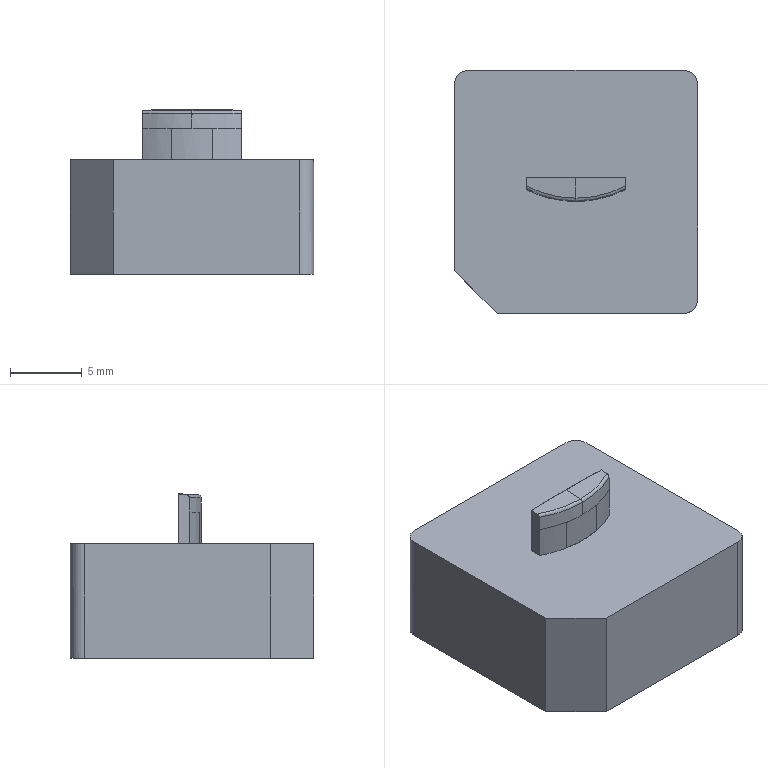NC program | PowerMill | posted with a generic post | part box 17 x 17 x 11.498 mm
Lines 2037 to 3902 of 31087, first 1642 of 1866 lines:
N2134 M6
N2135 S18000 M03
N2136 G00 G90 X0.0 Y0.0
N2137 G43 Z9.7979 H2
N2138
N2139 G05 P10000 R4
N2140 X-1.4386 Y3.9377
N2141 Z0.7981
N2142 G01 Z-0.4019 F3600.0
N2143 X-1.4484 Y3.918 F6000.0
N2144 G03 X-1.3599 Y3.6524 I0.1771 J-0.0885
N2145 G01 X0.0 Y2.9724
N2146 X3.1723
N2147 X3.6604 Y2.9618
N2148 X4.1484 Y2.848
N2149 X4.4884 Y2.6843
N2150 X4.6365 Y2.5854
N2151 X5.0359 Y2.1962
N2152 X5.1246 Y2.0722
N2153 X5.3138 Y1.7082
N2154 X5.4386 Y1.2201
N2155 X5.4548 Y0.244
N2156 X5.4013 Y-0.244
N2157 X5.2178 Y-0.7321
N2158 X5.1246 Y-0.89
N2159 X4.852 Y-1.2201
N2160 X4.6365 Y-1.4029
N2161 X4.1484 Y-1.6736
N2162 X3.6604 Y-1.8871
N2163 X2.7944 Y-2.1962
N2164 X2.1962 Y-2.3549
N2165 X1.7082 Y-2.4558
N2166 X0.7321 Y-2.5782
N2167 X-0.244 Y-2.6041
N2168 X-1.2201 Y-2.5297
N2169 X-2.1962 Y-2.3537
N2170 X-3.1723 Y-2.0713
N2171 X-4.0749 Y-1.7082
N2172 X-4.6365 Y-1.4029
N2173 X-4.852 Y-1.2201
N2174 X-5.1246 Y-0.89
N2175 X-5.2178 Y-0.7321
N2176 X-5.4013 Y-0.244
N2177 X-5.4548 Y0.244
N2178 X-5.4386 Y1.2201
N2179 X-5.3138 Y1.7082
N2180 X-5.1246 Y2.0722
N2181 X-5.0359 Y2.1962
N2182 X-4.6365 Y2.5854
N2183 X-4.4884 Y2.6843
N2184 X-4.1484 Y2.848
N2185 X-3.6604 Y2.9618
N2186 X-3.1723 Y2.9724
N2187 X0.0
N2188 X-1.4386 Y3.9377 Z-0.5918
N2189 X-1.4484 Y3.918
N2190 G03 X-1.3599 Y3.6524 I0.1771 J-0.0885
N2191 G01 X0.0 Y2.9724
N2192 X3.1723
N2193 X3.6604 Y2.9618
N2194 X4.1484 Y2.848
N2195 X4.4884 Y2.6843
N2196 X4.6365 Y2.5854
N2197 X5.0359 Y2.1962
N2198 X5.1246 Y2.0723
N2199 X5.3138 Y1.7082
N2200 X5.4387 Y1.2201
N2201 X5.4548 Y0.244
N2202 X5.4054 Y-0.244
N2203 X5.2275 Y-0.7321
N2204 X5.1246 Y-0.9098
N2205 X4.8736 Y-1.2201
N2206 X4.6365 Y-1.4248
N2207 X4.1484 Y-1.6942
N2208 X3.6604 Y-1.9098
N2209 X2.8607 Y-2.1962
N2210 X1.7082 Y-2.4809
N2211 X0.7321 Y-2.605
N2212 X-0.244 Y-2.6289
N2213 X-1.2201 Y-2.5538
N2214 X-2.1962 Y-2.3796
N2215 X-3.1723 Y-2.0983
N2216 X-4.1201 Y-1.7082
N2217 X-4.6365 Y-1.4248
N2218 X-4.8736 Y-1.2201
N2219 X-5.1246 Y-0.9098
N2220 X-5.2275 Y-0.7321
N2221 X-5.4054 Y-0.244
N2222 X-5.4548 Y0.244
N2223 X-5.4387 Y1.2201
N2224 X-5.3138 Y1.7082
N2225 X-5.1246 Y2.0723
N2226 X-5.0359 Y2.1962
N2227 X-4.6365 Y2.5854
N2228 X-4.4884 Y2.6843
N2229 X-4.1484 Y2.848
N2230 X-3.6604 Y2.9618
N2231 X-3.1723 Y2.9724
N2232 X0.0
N2233 X-1.4386 Y3.9377 Z-0.7817
N2234 X-1.4484 Y3.918
N2235 G03 X-1.3599 Y3.6524 I0.1771 J-0.0885
N2236 G01 X0.0 Y2.9725
N2237 X3.1723
N2238 X3.6604 Y2.9618
N2239 X4.1484 Y2.848
N2240 X4.4884 Y2.6843
N2241 X4.6365 Y2.5854
N2242 X5.0359 Y2.1962
N2243 X5.1246 Y2.0723
N2244 X5.3138 Y1.7082
N2245 X5.4387 Y1.2201
N2246 X5.4548 Y0.244
N2247 X5.4084 Y-0.244
N2248 X5.2325 Y-0.7321
N2249 X5.1246 Y-0.919
N2250 X4.8815 Y-1.2201
N2251 X4.6365 Y-1.4323
N2252 X4.1484 Y-1.7022
N2253 X3.6604 Y-1.9188
N2254 X2.8763 Y-2.1962
N2255 X2.6843 Y-2.2555
N2256 X1.7082 Y-2.4878
N2257 X0.7321 Y-2.6129
N2258 X0.244 Y-2.6332
N2259 X0.0001 Y-2.6253
N2260 X-0.244 Y-2.6288
N2261 X-0.3653 Y-2.6195
N2262 X-0.3706 Y-2.6194
N2263 X-0.7321 Y-2.6113
N2264 X-1.1344 Y-2.5604
N2265 X-1.2188 Y-2.554
N2266 X-1.302 Y-2.5392
N2267 X-1.7082 Y-2.4878
N2268 X-2.1962 Y-2.3842
N2269 X-3.1723 Y-2.1053
N2270 X-4.1354 Y-1.7082
N2271 X-4.6365 Y-1.4323
N2272 X-4.8815 Y-1.2201
N2273 X-5.1246 Y-0.919
N2274 X-5.2325 Y-0.7321
N2275 X-5.4084 Y-0.244
N2276 X-5.4548 Y0.244
N2277 X-5.4387 Y1.2201
N2278 X-5.3138 Y1.7082
N2279 X-5.1246 Y2.0723
N2280 X-5.0359 Y2.1962
N2281 X-4.6365 Y2.5854
N2282 X-4.4884 Y2.6843
N2283 X-4.1484 Y2.848
N2284 X-3.6604 Y2.9618
N2285 X-3.1723 Y2.9725
N2286 X0.0
N2287 X-1.4386 Y3.9377 Z-0.9715
N2288 X-1.4484 Y3.918
N2289 G03 X-1.3599 Y3.6524 I0.1771 J-0.0885
N2290 G01 X0.0 Y2.9725
N2291 X3.1723
N2292 X3.6604 Y2.9618
N2293 X4.1484 Y2.848
N2294 X4.4884 Y2.6843
N2295 X4.6365 Y2.5854
N2296 X5.0359 Y2.1962
N2297 X5.1246 Y2.0723
N2298 X5.3138 Y1.7082
N2299 X5.4387 Y1.2201
N2300 X5.4548 Y0.244
N2301 X5.41 Y-0.244
N2302 X5.2374 Y-0.7321
N2303 X5.1246 Y-0.9264
N2304 X4.8886 Y-1.2201
N2305 X4.6365 Y-1.4397
N2306 X4.1512 Y-1.7082
N2307 X3.6604 Y-1.9256
N2308 X2.899 Y-2.1962
N2309 X2.6843 Y-2.2629
N2310 X1.7082 Y-2.4946
N2311 X0.7321 Y-2.6196
N2312 X0.244 Y-2.6407
N2313 X-0.7321 Y-2.6183
N2314 X-1.7082 Y-2.4947
N2315 X-2.1962 Y-2.3909
N2316 X-3.1723 Y-2.1123
N2317 X-4.1507 Y-1.7082
N2318 X-4.6365 Y-1.4397
N2319 X-4.8886 Y-1.2201
N2320 X-5.1246 Y-0.9264
N2321 X-5.2374 Y-0.7321
N2322 X-5.41 Y-0.244
N2323 X-5.4548 Y0.244
N2324 X-5.4387 Y1.2201
N2325 X-5.3138 Y1.7082
N2326 X-5.1246 Y2.0723
N2327 X-5.0359 Y2.1962
N2328 X-4.6365 Y2.5854
N2329 X-4.4884 Y2.6843
N2330 X-4.1484 Y2.848
N2331 X-3.6604 Y2.9618
N2332 X-3.1723 Y2.9725
N2333 X0.0
N2334 X-1.4386 Y3.9377 Z-1.1614
N2335 X-1.4484 Y3.918
N2336 G03 X-1.3599 Y3.6524 I0.1771 J-0.0885
N2337 G01 X0.0 Y2.9725
N2338 X3.1723
N2339 X3.6604 Y2.9618
N2340 X4.1484 Y2.848
N2341 X4.4884 Y2.6843
N2342 X4.6365 Y2.5854
N2343 X5.0359 Y2.1962
N2344 X5.1246 Y2.0723
N2345 X5.3138 Y1.7082
N2346 X5.4387 Y1.2201
N2347 X5.4548 Y0.244
N2348 X5.4116 Y-0.244
N2349 X5.2411 Y-0.7321
N2350 X5.1246 Y-0.9339
N2351 X4.8958 Y-1.2201
N2352 X4.6365 Y-1.4471
N2353 X4.167 Y-1.7082
N2354 X3.6604 Y-1.9325
N2355 X2.9221 Y-2.1962
N2356 X2.6843 Y-2.2704
N2357 X1.7082 Y-2.5015
N2358 X0.7321 Y-2.6262
N2359 X0.244 Y-2.6482
N2360 X-0.7321 Y-2.6254
N2361 X-1.7082 Y-2.5015
N2362 X-2.1962 Y-2.3978
N2363 X-3.1723 Y-2.1193
N2364 X-4.1484 Y-1.7168
N2365 X-4.6365 Y-1.4471
N2366 X-4.8958 Y-1.2201
N2367 X-5.1246 Y-0.9339
N2368 X-5.2411 Y-0.7321
N2369 X-5.4116 Y-0.244
N2370 X-5.4548 Y0.244
N2371 X-5.4387 Y1.2201
N2372 X-5.3138 Y1.7082
N2373 X-5.1246 Y2.0723
N2374 X-5.0359 Y2.1962
N2375 X-4.6365 Y2.5854
N2376 X-4.4884 Y2.6843
N2377 X-4.1484 Y2.848
N2378 X-3.6604 Y2.9618
N2379 X-3.1723 Y2.9725
N2380 X0.0
N2381 X-1.4386 Y3.9377 Z-1.3513
N2382 X-1.4484 Y3.918
N2383 G03 X-1.3599 Y3.6524 I0.1771 J-0.0885
N2384 G01 X0.0 Y2.9725
N2385 X3.1723
N2386 X3.6604 Y2.9618
N2387 X4.1484 Y2.848
N2388 X4.4884 Y2.6843
N2389 X4.6365 Y2.5855
N2390 X5.036 Y2.1962
N2391 X5.1246 Y2.0723
N2392 X5.3138 Y1.7082
N2393 X5.4387 Y1.2201
N2394 X5.4548 Y0.244
N2395 X5.4131 Y-0.244
N2396 X5.2449 Y-0.7321
N2397 X5.1246 Y-0.9413
N2398 X4.9029 Y-1.2201
N2399 X4.6365 Y-1.4545
N2400 X4.1828 Y-1.7082
N2401 X3.6604 Y-1.9394
N2402 X2.9463 Y-2.1962
N2403 X2.6843 Y-2.2778
N2404 X1.7082 Y-2.5084
N2405 X1.2201 Y-2.5815
N2406 X0.8795 Y-2.6073
N2407 X0.7321 Y-2.6262
N2408 X0.4866 Y-2.6372
N2409 X0.4835 Y-2.6374
N2410 X0.244 Y-2.6557
N2411 X-0.7321 Y-2.6325
N2412 X-1.7082 Y-2.5084
N2413 X-2.1962 Y-2.4046
N2414 X-3.1723 Y-2.1262
N2415 X-4.1828 Y-1.7082
N2416 X-4.6365 Y-1.4545
N2417 X-4.9029 Y-1.2201
N2418 X-5.1246 Y-0.9413
N2419 X-5.2449 Y-0.7321
N2420 X-5.4131 Y-0.244
N2421 X-5.4548 Y0.244
N2422 X-5.4387 Y1.2201
N2423 X-5.3138 Y1.7082
N2424 X-5.1246 Y2.0723
N2425 X-5.036 Y2.1962
N2426 X-4.6365 Y2.5855
N2427 X-4.4884 Y2.6843
N2428 X-4.1484 Y2.848
N2429 X-3.6604 Y2.9618
N2430 X-3.1723 Y2.9725
N2431 X0.0
N2432 X-1.4386 Y3.9377 Z-1.5412
N2433 X-1.4484 Y3.9181
N2434 G03 X-1.3599 Y3.6524 I0.1771 J-0.0886
N2435 G01 X0.0 Y2.9725
N2436 X3.1723
N2437 X3.6604 Y2.9618
N2438 X4.1484 Y2.848
N2439 X4.4884 Y2.6843
N2440 X4.6365 Y2.5855
N2441 X5.036 Y2.1962
N2442 X5.1246 Y2.0723
N2443 X5.3138 Y1.7082
N2444 X5.4387 Y1.2201
N2445 X5.4548 Y0.244
N2446 X5.4142 Y-0.244
N2447 X5.2473 Y-0.7321
N2448 X5.1246 Y-0.9464
N2449 X4.9078 Y-1.2201
N2450 X4.6365 Y-1.4596
N2451 X4.1938 Y-1.7082
N2452 X3.6604 Y-1.9463
N2453 X2.9714 Y-2.1962
N2454 X2.6843 Y-2.2836
N2455 X1.7082 Y-2.5141
N2456 X1.451 Y-2.5469
N2457 X1.2866 Y-2.5739
N2458 X1.1206 Y-2.589
N2459 X0.7321 Y-2.6385
N2460 X0.3461 Y-2.6478
N2461 X0.24 Y-2.6557
N2462 X0.1337 Y-2.653
N2463 X-0.244 Y-2.6621
N2464 X-0.5986 Y-2.6356
N2465 X-0.7311 Y-2.6325
N2466 X-0.8626 Y-2.6158
N2467 X-1.2201 Y-2.5891
N2468 X-1.5521 Y-2.5282
N2469 X-1.7082 Y-2.5084
N2470 X-2.0065 Y-2.4449
N2471 X-2.0093 Y-2.4444
N2472 X-2.1962 Y-2.4101
N2473 X-3.1723 Y-2.1315
N2474 X-4.194 Y-1.7082
N2475 X-4.6365 Y-1.4596
N2476 X-4.9078 Y-1.2201
N2477 X-5.1246 Y-0.9464
N2478 X-5.2473 Y-0.7321
N2479 X-5.4142 Y-0.244
N2480 X-5.4548 Y0.244
N2481 X-5.4387 Y1.2201
N2482 X-5.3138 Y1.7082
N2483 X-5.1246 Y2.0723
N2484 X-5.036 Y2.1962
N2485 X-4.6365 Y2.5855
N2486 X-4.4884 Y2.6843
N2487 X-4.1484 Y2.848
N2488 X-3.6604 Y2.9618
N2489 X-3.1723 Y2.9725
N2490 X0.0
N2491 X-1.4386 Y3.9377 Z-1.7311
N2492 X-1.4484 Y3.9181
N2493 G03 X-1.3599 Y3.6524 I0.1771 J-0.0886
N2494 G01 X0.0 Y2.9725
N2495 X3.1723
N2496 X3.6604 Y2.9618
N2497 X4.1484 Y2.848
N2498 X4.4884 Y2.6843
N2499 X4.6365 Y2.5855
N2500 X5.036 Y2.1962
N2501 X5.1246 Y2.0723
N2502 X5.3138 Y1.7082
N2503 X5.4387 Y1.2201
N2504 X5.4548 Y0.244
N2505 X5.4142 Y-0.244
N2506 X5.2473 Y-0.7321
N2507 X5.1246 Y-0.9465
N2508 X4.9079 Y-1.2201
N2509 X4.6365 Y-1.4596
N2510 X4.1939 Y-1.7082
N2511 X3.6604 Y-1.947
N2512 X2.9714 Y-2.1962
N2513 X2.6843 Y-2.2837
N2514 X1.7082 Y-2.5141
N2515 X1.4483 Y-2.5472
N2516 X1.2858 Y-2.574
N2517 X1.1218 Y-2.5888
N2518 X0.7321 Y-2.6385
N2519 X0.345 Y-2.6479
N2520 X0.2401 Y-2.6557
N2521 X0.1349 Y-2.653
N2522 X-0.244 Y-2.6621
N2523 X-0.5998 Y-2.6355
N2524 X-0.7311 Y-2.6324
N2525 X-0.8615 Y-2.6159
N2526 X-1.2201 Y-2.5891
N2527 X-1.5532 Y-2.528
N2528 X-1.5586 Y-2.5273
N2529 X-1.7082 Y-2.5083
N2530 X-1.9515 Y-2.4558
N2531 X-2.1962 Y-2.4101
N2532 X-3.1723 Y-2.1315
N2533 X-3.6604 Y-1.9456
N2534 X-4.194 Y-1.7082
N2535 X-4.6365 Y-1.4596
N2536 X-4.9079 Y-1.2201
N2537 X-5.1246 Y-0.9465
N2538 X-5.2473 Y-0.7321
N2539 X-5.4142 Y-0.244
N2540 X-5.4548 Y0.244
N2541 X-5.4387 Y1.2201
N2542 X-5.3138 Y1.7082
N2543 X-5.1246 Y2.0723
N2544 X-5.036 Y2.1962
N2545 X-4.6365 Y2.5855
N2546 X-4.4884 Y2.6843
N2547 X-4.1484 Y2.848
N2548 X-3.6604 Y2.9618
N2549 X-3.1723 Y2.9725
N2550 X0.0
N2551 X-1.4386 Y3.9377 Z-1.921
N2552 X-1.4484 Y3.9181
N2553 G03 X-1.3599 Y3.6524 I0.1771 J-0.0886
N2554 G01 X0.0 Y2.9725
N2555 X3.1723
N2556 X3.6604 Y2.9618
N2557 X4.1484 Y2.848
N2558 X4.4884 Y2.6843
N2559 X4.6365 Y2.5855
N2560 X5.036 Y2.1962
N2561 X5.1246 Y2.0723
N2562 X5.3138 Y1.7082
N2563 X5.4387 Y1.2201
N2564 X5.4548 Y0.244
N2565 X5.4142 Y-0.244
N2566 X5.2473 Y-0.7321
N2567 X5.1246 Y-0.9465
N2568 X4.9079 Y-1.2201
N2569 X4.6365 Y-1.4596
N2570 X4.1939 Y-1.7082
N2571 X3.6604 Y-1.9472
N2572 X2.9714 Y-2.1962
N2573 X2.6843 Y-2.2837
N2574 X1.7082 Y-2.5141
N2575 X1.4456 Y-2.5476
N2576 X1.285 Y-2.574
N2577 X1.1229 Y-2.5887
N2578 X0.7321 Y-2.6385
N2579 X0.3438 Y-2.6479
N2580 X0.2401 Y-2.6556
N2581 X0.1361 Y-2.6529
N2582 X-0.244 Y-2.6621
N2583 X-0.6009 Y-2.6354
N2584 X-0.7311 Y-2.6324
N2585 X-0.8604 Y-2.616
N2586 X-1.2201 Y-2.5891
N2587 X-1.5543 Y-2.5278
N2588 X-1.5596 Y-2.5271
N2589 X-1.7082 Y-2.5083
N2590 X-1.9515 Y-2.4558
N2591 X-2.1962 Y-2.4101
N2592 X-3.1723 Y-2.1316
N2593 X-3.6604 Y-1.946
N2594 X-4.194 Y-1.7082
N2595 X-4.6365 Y-1.4596
N2596 X-4.9079 Y-1.2201
N2597 X-5.1246 Y-0.9465
N2598 X-5.2473 Y-0.7321
N2599 X-5.4142 Y-0.244
N2600 X-5.4548 Y0.244
N2601 X-5.4387 Y1.2201
N2602 X-5.3138 Y1.7082
N2603 X-5.1246 Y2.0723
N2604 X-5.036 Y2.1962
N2605 X-4.6365 Y2.5855
N2606 X-4.4884 Y2.6843
N2607 X-4.1484 Y2.848
N2608 X-3.6604 Y2.9618
N2609 X-3.1723 Y2.9725
N2610 X0.0
N2611 X-1.4386 Y3.9377 Z-2.1109
N2612 X-1.4484 Y3.9181
N2613 G03 X-1.3598 Y3.6524 I0.1771 J-0.0886
N2614 G01 X0.0 Y2.9725
N2615 X3.1723
N2616 X3.6604 Y2.9618
N2617 X4.1484 Y2.848
N2618 X4.4884 Y2.6843
N2619 X4.6365 Y2.5855
N2620 X5.036 Y2.1962
N2621 X5.1246 Y2.0723
N2622 X5.3138 Y1.7082
N2623 X5.4387 Y1.2201
N2624 X5.4548 Y0.244
N2625 X5.4142 Y-0.244
N2626 X5.2474 Y-0.7321
N2627 X5.1246 Y-0.9465
N2628 X4.9079 Y-1.2201
N2629 X4.6365 Y-1.4596
N2630 X4.1939 Y-1.7082
N2631 X3.6604 Y-1.9472
N2632 X2.9714 Y-2.1962
N2633 X2.6843 Y-2.2837
N2634 X1.7082 Y-2.5141
N2635 X1.4429 Y-2.5479
N2636 X1.2842 Y-2.574
N2637 X1.1241 Y-2.5886
N2638 X0.7321 Y-2.6385
N2639 X0.3427 Y-2.648
N2640 X0.2402 Y-2.6556
N2641 X0.1374 Y-2.6529
N2642 X-0.244 Y-2.6621
N2643 X-0.6021 Y-2.6353
N2644 X-0.7311 Y-2.6323
N2645 X-0.8592 Y-2.6161
N2646 X-1.2201 Y-2.5891
N2647 X-1.5553 Y-2.5276
N2648 X-1.5607 Y-2.527
N2649 X-1.7082 Y-2.5082
N2650 X-1.9515 Y-2.4557
N2651 X-2.1962 Y-2.4102
N2652 X-3.1723 Y-2.1316
N2653 X-3.6604 Y-1.9464
N2654 X-4.194 Y-1.7082
N2655 X-4.6365 Y-1.4596
N2656 X-4.9079 Y-1.2201
N2657 X-5.1246 Y-0.9465
N2658 X-5.2474 Y-0.7321
N2659 X-5.4142 Y-0.244
N2660 X-5.4548 Y0.244
N2661 X-5.4387 Y1.2201
N2662 X-5.3138 Y1.7082
N2663 X-5.1246 Y2.0723
N2664 X-5.036 Y2.1962
N2665 X-4.6365 Y2.5855
N2666 X-4.4884 Y2.6843
N2667 X-4.1484 Y2.848
N2668 X-3.6604 Y2.9618
N2669 X-3.1723 Y2.9725
N2670 X0.0
N2671 X-1.4386 Y3.9377 Z-2.3008
N2672 X-1.4484 Y3.9181
N2673 G03 X-1.3598 Y3.6524 I0.1771 J-0.0886
N2674 G01 X0.0 Y2.9725
N2675 X3.1723
N2676 X3.6604 Y2.9618
N2677 X4.1484 Y2.8481
N2678 X4.4884 Y2.6843
N2679 X4.6365 Y2.5855
N2680 X5.036 Y2.1962
N2681 X5.1246 Y2.0723
N2682 X5.3138 Y1.7082
N2683 X5.4387 Y1.2201
N2684 X5.4548 Y0.244
N2685 X5.4142 Y-0.244
N2686 X5.2474 Y-0.7321
N2687 X5.1246 Y-0.9465
N2688 X4.9079 Y-1.2201
N2689 X4.6365 Y-1.4597
N2690 X4.1939 Y-1.7082
N2691 X3.6604 Y-1.9472
N2692 X2.9714 Y-2.1962
N2693 X2.7316 Y-2.2708
N2694 X2.4876 Y-2.3302
N2695 X2.1962 Y-2.4109
N2696 X1.9509 Y-2.4562
N2697 X1.7082 Y-2.514
N2698 X1.4631 Y-2.545
N2699 X1.2201 Y-2.5891
N2700 X0.9755 Y-2.6074
N2701 X0.7321 Y-2.6385
N2702 X0.4878 Y-2.6441
N2703 X0.244 Y-2.6619
N2704 X0.0 Y-2.6561
N2705 X-0.244 Y-2.6621
N2706 X-0.4878 Y-2.6441
N2707 X-0.7321 Y-2.6384
N2708 X-0.9755 Y-2.6074
N2709 X-1.2201 Y-2.589
N2710 X-1.4631 Y-2.5449
N2711 X-1.7082 Y-2.5141
N2712 X-1.951 Y-2.4564
N2713 X-2.1962 Y-2.4101
N2714 X-2.4388 Y-2.3417
N2715 X-2.6843 Y-2.285
N2716 X-2.9262 Y-2.2015
N2717 X-3.1723 Y-2.1315
N2718 X-3.6468 Y-1.9515
N2719 X-3.6604 Y-1.9468
N2720 X-4.194 Y-1.7082
N2721 X-4.6365 Y-1.4597
N2722 X-4.9079 Y-1.2201
N2723 X-5.1246 Y-0.9465
N2724 X-5.2474 Y-0.7321
N2725 X-5.4142 Y-0.244
N2726 X-5.4548 Y0.244
N2727 X-5.4387 Y1.2201
N2728 X-5.3138 Y1.7082
N2729 X-5.1246 Y2.0723
N2730 X-5.036 Y2.1962
N2731 X-4.6365 Y2.5855
N2732 X-4.4884 Y2.6843
N2733 X-4.1484 Y2.8481
N2734 X-3.6604 Y2.9618
N2735 X-3.1723 Y2.9725
N2736 X0.0
N2737 X-1.4386 Y3.9377 Z-2.4907
N2738 X-1.4484 Y3.9181
N2739 G03 X-1.3598 Y3.6524 I0.1771 J-0.0886
N2740 G01 X0.0 Y2.9725
N2741 X3.1723
N2742 X3.6604 Y2.9618
N2743 X4.1484 Y2.8481
N2744 X4.4884 Y2.6843
N2745 X4.6365 Y2.5855
N2746 X5.036 Y2.1962
N2747 X5.1246 Y2.0723
N2748 X5.3138 Y1.7082
N2749 X5.4387 Y1.2201
N2750 X5.4548 Y0.244
N2751 X5.4142 Y-0.244
N2752 X5.2474 Y-0.7321
N2753 X5.1246 Y-0.9465
N2754 X4.9079 Y-1.2201
N2755 X4.6365 Y-1.4597
N2756 X4.1939 Y-1.7082
N2757 X3.6604 Y-1.9472
N2758 X2.9714 Y-2.1962
N2759 X2.7348 Y-2.2699
N2760 X2.494 Y-2.3287
N2761 X2.1962 Y-2.4112
N2762 X1.9509 Y-2.4563
N2763 X1.7082 Y-2.514
N2764 X1.4631 Y-2.545
N2765 X1.2201 Y-2.5891
N2766 X0.9755 Y-2.6074
N2767 X0.7321 Y-2.6384
N2768 X0.4878 Y-2.6441
N2769 X0.244 Y-2.662
N2770 X0.0 Y-2.6561
N2771 X-0.244 Y-2.662
N2772 X-0.4878 Y-2.6441
N2773 X-0.7321 Y-2.6384
N2774 X-0.9755 Y-2.6074
N2775 X-1.2201 Y-2.589
N2776 X-1.4631 Y-2.5449
N2777 X-1.7082 Y-2.5141
N2778 X-1.951 Y-2.4563
N2779 X-2.1962 Y-2.4101
N2780 X-2.4388 Y-2.3419
N2781 X-2.6843 Y-2.2853
N2782 X-2.9262 Y-2.2016
N2783 X-3.1723 Y-2.1315
N2784 X-3.6372 Y-1.9551
N2785 X-3.6604 Y-1.947
N2786 X-4.194 Y-1.7082
N2787 X-4.6365 Y-1.4597
N2788 X-4.9079 Y-1.2201
N2789 X-5.1246 Y-0.9465
N2790 X-5.2474 Y-0.7321
N2791 X-5.4142 Y-0.244
N2792 X-5.4548 Y0.244
N2793 X-5.4387 Y1.2201
N2794 X-5.3138 Y1.7082
N2795 X-5.1246 Y2.0723
N2796 X-5.036 Y2.1962
N2797 X-4.6365 Y2.5855
N2798 X-4.4884 Y2.6843
N2799 X-4.1484 Y2.8481
N2800 X-3.6604 Y2.9618
N2801 X-3.1723 Y2.9725
N2802 X0.0
N2803 X-1.4386 Y3.9378 Z-2.6806
N2804 X-1.4484 Y3.9181
N2805 G03 X-1.3598 Y3.6524 I0.1771 J-0.0886
N2806 G01 X0.0 Y2.9725
N2807 X3.1723
N2808 X3.6604 Y2.9618
N2809 X4.1484 Y2.8481
N2810 X4.4884 Y2.6843
N2811 X4.6365 Y2.5855
N2812 X5.036 Y2.1962
N2813 X5.1246 Y2.0723
N2814 X5.3138 Y1.7082
N2815 X5.4387 Y1.2201
N2816 X5.4548 Y0.244
N2817 X5.4142 Y-0.244
N2818 X5.2474 Y-0.7321
N2819 X5.1246 Y-0.9465
N2820 X4.9079 Y-1.2201
N2821 X4.6365 Y-1.4597
N2822 X4.1939 Y-1.7082
N2823 X3.6604 Y-1.9472
N2824 X2.9714 Y-2.1962
N2825 X2.7379 Y-2.269
N2826 X2.5002 Y-2.3271
N2827 X2.1962 Y-2.4116
N2828 X1.9509 Y-2.4564
N2829 X1.7082 Y-2.5139
N2830 X1.4631 Y-2.545
N2831 X1.2201 Y-2.5891
N2832 X0.9755 Y-2.6074
N2833 X0.7321 Y-2.6384
N2834 X0.4878 Y-2.644
N2835 X0.244 Y-2.662
N2836 X0.0 Y-2.6561
N2837 X-0.244 Y-2.662
N2838 X-0.4878 Y-2.644
N2839 X-0.7321 Y-2.6385
N2840 X-0.9755 Y-2.6074
N2841 X-1.2201 Y-2.5889
N2842 X-1.4631 Y-2.5449
N2843 X-1.7082 Y-2.5141
N2844 X-1.9509 Y-2.4562
N2845 X-2.1962 Y-2.41
N2846 X-2.4388 Y-2.342
N2847 X-2.6843 Y-2.2857
N2848 X-2.9261 Y-2.2017
N2849 X-3.1723 Y-2.1314
N2850 X-3.6348 Y-1.956
N2851 X-3.6604 Y-1.9471
N2852 X-4.194 Y-1.7082
N2853 X-4.6365 Y-1.4597
N2854 X-4.9079 Y-1.2201
N2855 X-5.1246 Y-0.9465
N2856 X-5.2474 Y-0.7321
N2857 X-5.4142 Y-0.244
N2858 X-5.4548 Y0.244
N2859 X-5.4387 Y1.2201
N2860 X-5.3138 Y1.7082
N2861 X-5.1246 Y2.0723
N2862 X-5.036 Y2.1962
N2863 X-4.6365 Y2.5855
N2864 X-4.4884 Y2.6843
N2865 X-4.1484 Y2.8481
N2866 X-3.6604 Y2.9618
N2867 X-3.1723 Y2.9725
N2868 X0.0
N2869 X-1.4386 Y3.9378 Z-2.8704
N2870 X-1.4484 Y3.9181
N2871 G03 X-1.3598 Y3.6524 I0.1771 J-0.0886
N2872 G01 X0.0 Y2.9725
N2873 X3.1723
N2874 X3.6604 Y2.9618
N2875 X4.1484 Y2.8481
N2876 X4.4884 Y2.6843
N2877 X4.6365 Y2.5855
N2878 X5.036 Y2.1962
N2879 X5.1246 Y2.0723
N2880 X5.3138 Y1.7082
N2881 X5.4387 Y1.2201
N2882 X5.4549 Y0.244
N2883 X5.4142 Y-0.244
N2884 X5.2474 Y-0.7321
N2885 X5.1246 Y-0.9465
N2886 X4.9079 Y-1.2201
N2887 X4.6365 Y-1.4597
N2888 X4.1939 Y-1.7082
N2889 X3.6604 Y-1.9472
N2890 X2.9714 Y-2.1962
N2891 X2.4663 Y-2.3411
N2892 X1.9536 Y-2.456
N2893 X1.7081 Y-2.5139
N2894 X1.4631 Y-2.5451
N2895 X1.2201 Y-2.5891
N2896 X0.9755 Y-2.6073
N2897 X0.7321 Y-2.6383
N2898 X0.4877 Y-2.644
N2899 X0.244 Y-2.662
N2900 X0.0 Y-2.6561
N2901 X-0.244 Y-2.6619
N2902 X-0.4878 Y-2.644
N2903 X-0.7321 Y-2.6385
N2904 X-0.9754 Y-2.6073
N2905 X-1.2201 Y-2.5889
N2906 X-1.4631 Y-2.5448
N2907 X-1.7082 Y-2.5141
N2908 X-2.1972 Y-2.404
N2909 X-2.6843 Y-2.286
N2910 X-2.9261 Y-2.2018
N2911 X-3.1723 Y-2.1314
N2912 X-3.6323 Y-1.9568
N2913 X-3.635 Y-1.9559
N2914 X-3.6604 Y-1.9471
N2915 X-4.194 Y-1.7082
N2916 X-4.6365 Y-1.4597
N2917 X-4.9079 Y-1.2201
N2918 X-5.1246 Y-0.9465
N2919 X-5.2474 Y-0.7321
N2920 X-5.4142 Y-0.244
N2921 X-5.4549 Y0.244
N2922 X-5.4387 Y1.2201
N2923 X-5.3138 Y1.7082
N2924 X-5.1246 Y2.0723
N2925 X-5.036 Y2.1962
N2926 X-4.6365 Y2.5855
N2927 X-4.4884 Y2.6843
N2928 X-4.1484 Y2.8481
N2929 X-3.6604 Y2.9618
N2930 X-3.1723 Y2.9725
N2931 X0.0
N2932 X-1.4385 Y3.9378 Z-3.0603
N2933 X-1.4484 Y3.9181
N2934 G03 X-1.3598 Y3.6524 I0.1771 J-0.0886
N2935 G01 X0.0 Y2.9725
N2936 X3.1723
N2937 X3.6604 Y2.9618
N2938 X4.1484 Y2.8481
N2939 X4.4884 Y2.6843
N2940 X4.6365 Y2.5855
N2941 X5.036 Y2.1962
N2942 X5.1246 Y2.0723
N2943 X5.3139 Y1.7082
N2944 X5.4387 Y1.2201
N2945 X5.4549 Y0.244
N2946 X5.4143 Y-0.244
N2947 X5.2474 Y-0.7321
N2948 X5.1246 Y-0.9465
N2949 X4.9079 Y-1.2201
N2950 X4.6365 Y-1.4597
N2951 X4.1939 Y-1.7082
N2952 X3.6604 Y-1.9472
N2953 X2.9714 Y-2.1962
N2954 X2.4655 Y-2.3413
N2955 X1.9518 Y-2.4563
N2956 X1.7081 Y-2.5138
N2957 X1.4631 Y-2.545
N2958 X1.2201 Y-2.5891
N2959 X0.9755 Y-2.6073
N2960 X0.7321 Y-2.6383
N2961 X0.4877 Y-2.644
N2962 X0.244 Y-2.662
N2963 X0.0 Y-2.656
N2964 X-0.244 Y-2.6619
N2965 X-0.4878 Y-2.644
N2966 X-0.7321 Y-2.6385
N2967 X-0.9754 Y-2.6073
N2968 X-1.2201 Y-2.5888
N2969 X-1.4631 Y-2.5448
N2970 X-1.7082 Y-2.5141
N2971 X-2.1971 Y-2.404
N2972 X-2.6843 Y-2.2863
N2973 X-2.9261 Y-2.2019
N2974 X-3.1723 Y-2.1313
N2975 X-3.6299 Y-1.9577
N2976 X-3.6325 Y-1.9568
N2977 X-3.6604 Y-1.9471
N2978 X-4.194 Y-1.7082
N2979 X-4.6365 Y-1.4597
N2980 X-4.9079 Y-1.2201
N2981 X-5.1246 Y-0.9465
N2982 X-5.2474 Y-0.7321
N2983 X-5.4143 Y-0.244
N2984 X-5.4549 Y0.244
N2985 X-5.4387 Y1.2201
N2986 X-5.3139 Y1.7082
N2987 X-5.1246 Y2.0723
N2988 X-5.036 Y2.1962
N2989 X-4.6365 Y2.5855
N2990 X-4.4884 Y2.6843
N2991 X-4.1484 Y2.8481
N2992 X-3.6604 Y2.9618
N2993 X-3.1723 Y2.9725
N2994 X0.0
N2995 X-1.4385 Y3.9378 Z-3.2502
N2996 X-1.4484 Y3.9181
N2997 G03 X-1.3598 Y3.6524 I0.1771 J-0.0886
N2998 G01 X0.0 Y2.9725
N2999 X3.1723
N3000 X3.6604 Y2.9618
N3001 X4.1484 Y2.8481
N3002 X4.4884 Y2.6843
N3003 X4.6365 Y2.5855
N3004 X5.036 Y2.1962
N3005 X5.1246 Y2.0723
N3006 X5.3139 Y1.7082
N3007 X5.4387 Y1.2201
N3008 X5.4549 Y0.244
N3009 X5.4143 Y-0.244
N3010 X5.2474 Y-0.7321
N3011 X5.1246 Y-0.9465
N3012 X4.9079 Y-1.2201
N3013 X4.6365 Y-1.4597
N3014 X4.1939 Y-1.7082
N3015 X3.6604 Y-1.9472
N3016 X2.9715 Y-2.1962
N3017 X2.4648 Y-2.3415
N3018 X1.9505 Y-2.4566
N3019 X1.7081 Y-2.5138
N3020 X1.4631 Y-2.545
N3021 X1.2201 Y-2.5891
N3022 X0.9755 Y-2.6073
N3023 X0.7321 Y-2.6382
N3024 X0.4877 Y-2.644
N3025 X0.244 Y-2.662
N3026 X0.0 Y-2.656
N3027 X-0.244 Y-2.6618
N3028 X-0.4878 Y-2.644
N3029 X-0.7321 Y-2.6385
N3030 X-0.9754 Y-2.6073
N3031 X-1.2201 Y-2.5888
N3032 X-1.4631 Y-2.5448
N3033 X-1.7082 Y-2.5141
N3034 X-2.1971 Y-2.404
N3035 X-2.6843 Y-2.2865
N3036 X-2.9261 Y-2.202
N3037 X-3.1722 Y-2.1313
N3038 X-3.6275 Y-1.9586
N3039 X-3.6301 Y-1.9577
N3040 X-3.6604 Y-1.9471
N3041 X-4.194 Y-1.7082
N3042 X-4.6365 Y-1.4597
N3043 X-4.9079 Y-1.2201
N3044 X-5.1246 Y-0.9465
N3045 X-5.2474 Y-0.7321
N3046 X-5.4143 Y-0.244
N3047 X-5.4549 Y0.244
N3048 X-5.4387 Y1.2201
N3049 X-5.3139 Y1.7082
N3050 X-5.1246 Y2.0723
N3051 X-5.036 Y2.1962
N3052 X-4.6365 Y2.5855
N3053 X-4.4884 Y2.6843
N3054 X-4.1484 Y2.8481
N3055 X-3.6604 Y2.9618
N3056 X-3.1723 Y2.9725
N3057 X0.0
N3058 X-1.4385 Y3.9378 Z-3.4401
N3059 X-1.4484 Y3.9181
N3060 G03 X-1.3598 Y3.6525 I0.1771 J-0.0886
N3061 G01 X0.0 Y2.9725
N3062 X3.1723
N3063 X3.6604 Y2.9619
N3064 X4.1484 Y2.8481
N3065 X4.4884 Y2.6843
N3066 X4.6365 Y2.5855
N3067 X5.036 Y2.1962
N3068 X5.1246 Y2.0723
N3069 X5.3139 Y1.7082
N3070 X5.4387 Y1.2201
N3071 X5.4549 Y0.244
N3072 X5.4143 Y-0.244
N3073 X5.2474 Y-0.7321
N3074 X5.1246 Y-0.9465
N3075 X4.9079 Y-1.2201
N3076 X4.6365 Y-1.4597
N3077 X4.1939 Y-1.7082
N3078 X3.6604 Y-1.9472
N3079 X2.9715 Y-2.1962
N3080 X2.9568 Y-2.2003
N3081 X2.9545 Y-2.201
N3082 X2.4556 Y-2.3439
N3083 X1.9491 Y-2.4569
N3084 X1.7081 Y-2.5137
N3085 X1.4631 Y-2.545
N3086 X1.2201 Y-2.5891
N3087 X0.9755 Y-2.6073
N3088 X0.7321 Y-2.6382
N3089 X0.4877 Y-2.644
N3090 X0.244 Y-2.662
N3091 X0.0 Y-2.656
N3092 X-0.244 Y-2.6618
N3093 X-0.4878 Y-2.644
N3094 X-0.7321 Y-2.6385
N3095 X-0.9754 Y-2.6073
N3096 X-1.2201 Y-2.5887
N3097 X-1.4631 Y-2.5448
N3098 X-1.7082 Y-2.5142
N3099 X-2.1971 Y-2.4041
N3100 X-2.6843 Y-2.2867
N3101 X-2.9261 Y-2.202
N3102 X-3.1722 Y-2.1312
N3103 X-3.6251 Y-1.9594
N3104 X-3.6604 Y-1.9471
N3105 X-4.194 Y-1.7082
N3106 X-4.6365 Y-1.4597
N3107 X-4.9079 Y-1.2201
N3108 X-5.1246 Y-0.9465
N3109 X-5.2474 Y-0.7321
N3110 X-5.4143 Y-0.244
N3111 X-5.4549 Y0.244
N3112 X-5.4387 Y1.2201
N3113 X-5.3139 Y1.7082
N3114 X-5.1246 Y2.0723
N3115 X-5.036 Y2.1962
N3116 X-4.6365 Y2.5855
N3117 X-4.4884 Y2.6843
N3118 X-4.1484 Y2.8481
N3119 X-3.6604 Y2.9619
N3120 X-3.1723 Y2.9725
N3121 X0.0
N3122 G00 Z2.8627
N3123 G01 X11.22 Y1.3157 F10000.0
N3124 G00 Z-2.43
N3125 G01 Z-3.63 F3600.0
N3126 X11.0 Y1.312 F6000.0
N3127 X5.4387 Y1.2201
N3128 X5.4549 Y0.244
N3129 X5.4143 Y-0.244
N3130 X5.2474 Y-0.7321
N3131 X5.1246 Y-0.9465
N3132 X4.9079 Y-1.2201
N3133 X4.6365 Y-1.4597
N3134 X4.194 Y-1.7082
N3135 X3.9241 Y-1.8291
N3136 X4.9894 Y-3.5111
N3137 X5.9745 Y-5.0667
N3138 X5.9161 Y-5.1037
N3139 G02 X1.0588 Y-6.4148 I-4.5411 J7.1705
N3140 G01 X-0.768 Y-6.3432
N3141 X-2.4386 Y-6.2062
N3142 G02 X-6.1515 Y-5.1372 I0.8298 J9.8648
N3143 G01 X-6.3816 Y-5.0184
N3144 G03 X-7.2288 Y-5.5926 I-0.2673 J-0.5176
N3145 G01 X-7.1471 Y-6.4287
N3146 G03 X-6.3509 Y-7.1509 I0.7962 J0.0778
N3147 G01 X6.352 Y-7.1507
N3148 G03 X7.1497 Y-6.4107 I0.0 J0.8
N3149 G01 X7.232 Y-5.3174
N3150 G03 X6.3833 Y-4.8079 I-0.5524 J0.0415
N3151 G01 X5.9745 Y-5.0667
N3152 X4.9894 Y-3.5111
N3153 G03 X6.7853 Y-1.7999 I-3.6219 J5.5991
N3154 G01 X7.3046 Y-1.0762
N3155 G02 X7.7444 Y-0.7708 I0.65 J-0.4664
N3156 G01 X8.0698 Y-0.6821
N3157 G02 X9.0801 Y-1.4545 I0.2103 J-0.7719
N3158 G01 X9.0754 Y-8.276
N3159 G02 X8.2754 Y-9.0754 I-0.8 J0.0006
N3160 G01 X-8.2754
N3161 G02 X-9.0754 Y-8.2754 I0.0 J0.8
N3162 G01 Y8.2754
N3163 G02 X-8.2754 Y9.0754 I0.8 J0.0
N3164 G01 X-0.6245
N3165 Y7.2754
N3166 X1.3816
N3167 G02 X1.3874 Y6.8755 I0.0 J-0.2
N3168 G01 X-2.6178 Y6.7598
N3169 G02 X-2.8234 Y6.9524 I-0.0058 J0.1999
N3170 G01 X-2.826 Y7.0054
N3171 X-2.8299 Y7.0583
N3172 G02 X-2.6307 Y7.2754 I0.1992 J0.0171
N3173 G01 X-0.6245
N3174 Y9.0754
N3175 X5.2752
N3176 X5.1263 Y7.2308
N3177 X6.4703 Y7.1223
N3178 X6.5988 Y7.0999
N3179 X6.721 Y7.0544
N3180 X6.8819 Y6.9769
N3181 G02 X7.1636 Y6.147 I-0.2664 J-0.5532
N3182 G02 X6.3286 Y5.881 I-0.5481 J0.2767
N3183 G01 X6.022 Y6.043
N3184 X5.6797 Y6.2133
N3185 X5.3293 Y6.3665
N3186 X4.9565 Y6.5186
N3187 G02 X5.1263 Y7.2308 I0.14 J0.343
N3188 G01 X5.2752 Y9.0754
N3189 X8.2754
N3190 G02 X9.0754 Y8.2746 I0.0 J-0.8
N3191 G01 X9.0709 Y3.9963
N3192 G02 X8.1821 Y3.2021 I-0.8 J0.0008
N3193 G01 X7.097 Y3.3232
N3194 X6.924 Y3.3623
N3195 X6.7638 Y3.4386
N3196 X5.5276 Y4.206
N3197 G03 X2.2167 Y5.0987 I-3.139 J-5.0561
N3198 G01 X-3.1777 Y4.9429
N3199 G03 X-5.3718 Y4.3011 I0.1305 J-4.5175
N3200 G01 X-6.2025 Y5.9589
N3201 X-6.388 Y5.866
N3202 G02 X-7.0188 Y6.8369 I-0.2609 J0.5208
N3203 G01 X-6.8654 Y6.963
N3204 G02 X-6.4676 Y7.1224 I0.4504 J-0.548
N3205 G01 X-5.0078 Y7.2311
N3206 G02 X-4.8583 Y6.5354 I0.0266 J-0.3582
N3207 G01 X-5.2224 Y6.4029
N3208 X-5.5621 Y6.268
N3209 X-5.8934 Y6.1138
N3210 X-6.2025 Y5.9589
N3211 X-5.3718 Y4.3011
N3212 G03 X-3.8168 Y-4.0279 I2.3246 J-3.8757
N3213 G01 X-1.8809 Y-4.3625
N3214 X-1.1471 Y-4.4643
N3215 X-0.4082 Y-4.5172
N3216 X1.1121 Y-4.5755
N3217 G03 X4.9894 Y-3.5111 I0.2554 J6.6635
N3218 G01 X3.9241 Y-1.8291
N3219 X3.6604 Y-1.9473
N3220 X2.9715 Y-2.1962
N3221 X2.9546 Y-2.2009
N3222 X2.6842 Y-2.2833
N3223 X2.5168 Y-2.3228
N3224 X2.1962 Y-2.412
N3225 X1.9478 Y-2.4571
N3226 X1.7081 Y-2.5137
N3227 X1.4656 Y-2.5446
N3228 X1.2201 Y-2.5892
N3229 X0.9696 Y-2.6079
N3230 X0.732 Y-2.6381
N3231 X0.4832 Y-2.6442
N3232 X0.244 Y-2.662
N3233 X-0.006 Y-2.656
N3234 X-0.244 Y-2.6617
N3235 X-0.4703 Y-2.6448
N3236 X-0.7321 Y-2.6385
N3237 X-0.9852 Y-2.6063
N3238 X-1.2201 Y-2.5887
N3239 X-1.4408 Y-2.5482
N3240 X-1.7082 Y-2.5142
N3241 X-2.0093 Y-2.444
N3242 X-2.1961 Y-2.4098
N3243 X-2.373 Y-2.3593
N3244 X-2.6843 Y-2.2868
N3245 X-2.9454 Y-2.1959
N3246 X-3.1722 Y-2.1312
N3247 X-3.6228 Y-1.9602
N3248 X-3.6604 Y-1.9471
N3249 X-4.1941 Y-1.7082
N3250 X-4.6365 Y-1.4597
N3251 X-4.9079 Y-1.2201
N3252 X-5.1246 Y-0.9465
N3253 X-5.2474 Y-0.7321
N3254 X-5.4143 Y-0.244
N3255 X-5.4549 Y0.244
N3256 X-5.4387 Y1.2201
N3257 X-5.3139 Y1.7082
N3258 X-5.1246 Y2.0723
N3259 X-5.036 Y2.1962
N3260 X-4.6365 Y2.5855
N3261 X-4.4885 Y2.6843
N3262 X-4.1484 Y2.8481
N3263 X-3.6604 Y2.9619
N3264 X-3.1723 Y2.9725
N3265 X3.1723
N3266 X3.6604 Y2.9619
N3267 X4.1484 Y2.8481
N3268 X4.4885 Y2.6843
N3269 X4.6365 Y2.5855
N3270 X5.036 Y2.1962
N3271 X5.1246 Y2.0723
N3272 X5.3139 Y1.7082
N3273 X5.4387 Y1.2201
N3274 X11.0 Y1.312
N3275 G00 Z9.7979
N3276 G05 P0
N3277 (---------------)
N3278 ( END TOOLPATH : 精公再粗02-外形偏置-D4C )
N3279 (---------------)
N3280
N3281 M05
N3282 G53 Z0.0
N3283 (---------------)
N3284 ( START TOOLPATH : 精公基准台01-基准面偏置-D10 )
N3285 (---------------)
N3286 ( TOOL NO.    :3 )
N3287 ( TOOL TYPE   : ENDMILL)
N3288 ( TOOL ID     : D10_1_1)
N3289 ( TOOL DIA    : 10.0 LENGTH 66.64)
N3290 T3
N3291 M6
N3292 S8500 M03
N3293 G00 G90 X0.0 Y0.0
N3294 G43 Z9.7979 H3
N3295
N3296 G05 P10000 R8
N3297 X17.6644 Y13.4005
N3298 Z-2.5
N3299 G01 Z-3.7 F360.0
N3300 X13.0549 Y10.8358 F600.0
N3301 X3.4681 Y6.3521
N3302 X3.7356 Y6.3451
N3303 X4.0164 Y6.323
N3304 X4.2957 Y6.2863
N3305 X4.5726 Y6.2349
N3306 X4.8465 Y6.1692
N3307 X5.1166 Y6.0892
N3308 X5.3821 Y5.9952
N3309 X5.6423 Y5.8874
N3310 X5.8965 Y5.7661
N3311 X6.1441 Y5.6317
N3312 X6.3842 Y5.4845
N3313 X6.6164 Y5.325
N3314 X6.8398 Y5.1535
N3315 X7.054 Y4.9706
N3316 X7.2583 Y4.7767
N3317 X7.4522 Y4.5724
N3318 X7.6351 Y4.3582
N3319 X7.8066 Y4.1348
N3320 X7.9661 Y3.9027
N3321 X8.1133 Y3.6625
N3322 X8.2477 Y3.415
N3323 X8.3689 Y3.1607
N3324 X8.4767 Y2.9005
N3325 X8.5708 Y2.635
N3326 X8.6508 Y2.3649
N3327 X8.7165 Y2.0911
N3328 X8.7678 Y1.8141
N3329 X8.8046 Y1.5349
N3330 X8.8267 Y1.2541
N3331 X8.8341 Y0.9725
N3332 Y0.1533
N3333 X8.8271 Y-0.1205
N3334 X8.8062 Y-0.3936
N3335 X8.7714 Y-0.6653
N3336 X8.7229 Y-0.9348
N3337 X8.6607 Y-1.2016
N3338 X8.585 Y-1.4648
N3339 X8.496 Y-1.7238
N3340 X8.3939 Y-1.978
N3341 X8.279 Y-2.2267
N3342 X8.1516 Y-2.4691
N3343 X8.0121 Y-2.7048
N3344 X7.8607 Y-2.9331
N3345 X7.6979 Y-3.1534
N3346 X7.5241 Y-3.3651
N3347 X7.3398 Y-3.5676
N3348 X7.1454 Y-3.7606
N3349 X6.9414 Y-3.9434
N3350 X6.7284 Y-4.1155
N3351 X6.5069 Y-4.2767
N3352 X6.2775 Y-4.4263
N3353 X6.0407 Y-4.564
N3354 G02 X4.7215 Y-5.163 I-5.7799 J10.9784
N3355 G01 X4.4177 Y-5.277
N3356 X4.1108 Y-5.3822
N3357 G02 X2.8421 Y-5.7329 I-4.1083 J12.3946
N3358 G01 X2.5857 Y-5.7878
N3359 X2.328 Y-5.836
N3360 X1.7729 Y-5.9254
N3361 X1.0669 Y-6.0026
N3362 X0.3562 Y-6.0414
N3363 X-0.3562
N3364 X-1.0669 Y-6.0026
N3365 X-1.773 Y-5.9254
N3366 X-2.3282 Y-5.836
N3367 X-2.5926 Y-5.7857
N3368 X-2.9357 Y-5.7114
N3369 X-3.1765 Y-5.6534
N3370 X-3.5181 Y-5.5628
N3371 X-3.7553 Y-5.494
N3372 X-4.0935 Y-5.3875
N3373 X-4.327 Y-5.308
N3374 X-4.6601 Y-5.186
N3375 X-4.8897 Y-5.0959
N3376 X-5.216 Y-4.9591
N3377 X-5.4414 Y-4.8585
N3378 X-5.7592 Y-4.7078
N3379 X-6.0053 Y-4.5833
N3380 X-6.2447 Y-4.4463
N3381 X-6.4767 Y-4.2973
N3382 X-6.7009 Y-4.1365
N3383 X-6.9165 Y-3.9645
N3384 X-7.123 Y-3.7816
N3385 X-7.3198 Y-3.5884
N3386 X-7.5065 Y-3.3854
N3387 X-7.6825 Y-3.173
N3388 X-7.8474 Y-2.9519
N3389 X-8.0008 Y-2.7227
N3390 X-8.1422 Y-2.4859
N3391 X-8.2713 Y-2.2421
N3392 X-8.3878 Y-1.9921
N3393 X-8.4913 Y-1.7364
N3394 X-8.5815 Y-1.4758
N3395 X-8.6582 Y-1.2109
N3396 X-8.7213 Y-0.9424
N3397 X-8.7705 Y-0.671
N3398 X-8.8058 Y-0.3974
N3399 X-8.827 Y-0.1224
N3400 X-8.8341 Y0.1533
N3401 Y0.9725
N3402 X-8.8267 Y1.2541
N3403 X-8.8046 Y1.5349
N3404 X-8.7678 Y1.8141
N3405 X-8.7165 Y2.0911
N3406 X-8.6508 Y2.3649
N3407 X-8.5708 Y2.635
N3408 X-8.4767 Y2.9005
N3409 X-8.3689 Y3.1607
N3410 X-8.2477 Y3.415
N3411 X-8.1133 Y3.6625
N3412 X-7.9661 Y3.9027
N3413 X-7.8066 Y4.1348
N3414 X-7.6351 Y4.3582
N3415 X-7.4522 Y4.5724
N3416 X-7.2583 Y4.7767
N3417 X-7.054 Y4.9706
N3418 X-6.8398 Y5.1535
N3419 X-6.6164 Y5.325
N3420 X-6.3842 Y5.4845
N3421 X-6.1441 Y5.6317
N3422 X-5.8965 Y5.7661
N3423 X-5.6423 Y5.8874
N3424 X-5.3821 Y5.9952
N3425 X-5.1166 Y6.0892
N3426 X-4.8465 Y6.1692
N3427 X-4.5726 Y6.2349
N3428 X-4.2957 Y6.2863
N3429 X-4.0164 Y6.323
N3430 X-3.7356 Y6.3451
N3431 X-3.4541 Y6.3525
N3432 X3.4681 Y6.3521
N3433 G00 Z9.7979
N3434 G05 P0
N3435 (---------------)
N3436 ( END TOOLPATH : 精公基准台01-基准面偏置-D10 )
N3437 (---------------)
N3438 ( START TOOLPATH : 精公基准台01-基准台侧光-D10 )
N3439 (---------------)
N3440 G00 X0.0 Y0.0 Z9.7979
N3441 G05 P10000 R8
N3442 X13.8128 Y-16.6019
N3443 Z-10.4
N3444 G01 Z-11.6 F360.0
N3445 G03 X10.9748 Y-12.4853 I-1.419 J2.0583 F600.0
N3446 G01 X10.7944 Y-12.6097
N3447 X10.7928 Y-12.6108
N3448 X10.7913 Y-12.6118
N3449 X10.6278 Y-12.7137
N3450 X10.6266 Y-12.7144
N3451 X10.6255 Y-12.715
N3452 X10.4729 Y-12.8035
N3453 X10.4714 Y-12.8043
N3454 X10.4698 Y-12.8052
N3455 X10.1537 Y-12.9703
N3456 X10.1516 Y-12.9713
N3457 X10.1495 Y-12.9723
N3458 X9.8333 Y-13.1144
N3459 X9.8312 Y-13.1153
N3460 X9.8291 Y-13.1162
N3461 X9.5129 Y-13.237
N3462 X9.5107 Y-13.2379
N3463 X9.5084 Y-13.2386
N3464 X9.1403 Y-13.3544
N3465 X9.1383 Y-13.3551
N3466 X9.1361 Y-13.3556
N3467 X8.8719 Y-13.4232
N3468 X8.8699 Y-13.4237
N3469 X8.8678 Y-13.4241
N3470 X8.5517 Y-13.4876
N3471 X8.5497 Y-13.488
N3472 X8.5478 Y-13.4883
N3473 X8.2317 Y-13.5357
N3474 X8.2294 Y-13.536
N3475 X8.2271 Y-13.5363
N3476 X7.911 Y-13.5653
N3477 X7.909 Y-13.5655
N3478 X7.9071 Y-13.5656
N3479 X7.5909 Y-13.5792
N3480 X7.5892
N3481 X7.5875
N3482 X-5.3745 Y-13.58
N3483 X-5.3749
N3484 X-5.3754
N3485 X-5.6915 Y-13.5764
N3486 X-5.6939 Y-13.5763
N3487 X-5.6962 Y-13.5762
N3488 X-6.0124 Y-13.5541
N3489 X-6.0149 Y-13.5538
N3490 X-6.0174 Y-13.5535
N3491 X-6.3336 Y-13.5111
N3492 X-6.3361 Y-13.5107
N3493 X-6.3386 Y-13.5103
N3494 X-6.6548 Y-13.447
N3495 X-6.6573 Y-13.4464
N3496 X-6.6598 Y-13.4458
N3497 X-6.976 Y-13.3608
N3498 X-6.9785 Y-13.3601
N3499 X-6.981 Y-13.3593
N3500 X-7.2972 Y-13.2514
N3501 X-7.2997 Y-13.2505
N3502 X-7.3022 Y-13.2495
N3503 X-7.6184 Y-13.1172
N3504 X-7.6203 Y-13.1163
N3505 X-7.6223 Y-13.1154
N3506 X-7.791 Y-13.034
N3507 X-7.7923 Y-13.0334
N3508 X-7.7936 Y-13.0328
N3509 X-7.9409 Y-12.9551
N3510 X-7.9428 Y-12.9541
N3511 X-7.9447 Y-12.953
N3512 X-8.2608 Y-12.7643
N3513 X-8.2624 Y-12.7633
N3514 X-8.2639 Y-12.7623
N3515 X-8.3391 Y-12.7126
N3516 X-8.3404 Y-12.7117
N3517 X-8.3417 Y-12.7108
N3518 X-8.5826 Y-12.5378
N3519 X-8.5843 Y-12.5365
N3520 X-8.5859 Y-12.5352
N3521 X-8.7646 Y-12.3921
N3522 X-8.7659 Y-12.3911
N3523 X-8.7671 Y-12.39
N3524 X-8.9046 Y-12.2703
N3525 X-8.906 Y-12.269
N3526 X-8.9074 Y-12.2678
N3527 X-9.1128 Y-12.0714
N3528 X-9.1135 Y-12.0707
N3529 X-9.1141 Y-12.0701
N3530 X-12.0701 Y-9.1141
N3531 X-12.0707 Y-9.1135
N3532 X-12.0714 Y-9.1128
N3533 X-12.2678 Y-8.9074
N3534 X-12.269 Y-8.906
N3535 X-12.2703 Y-8.9046
N3536 X-12.39 Y-8.7671
N3537 X-12.3911 Y-8.7659
N3538 X-12.3921 Y-8.7646
N3539 X-12.5352 Y-8.5859
N3540 X-12.5365 Y-8.5843
N3541 X-12.5378 Y-8.5826
N3542 X-12.7108 Y-8.3417
N3543 X-12.7117 Y-8.3404
N3544 X-12.7126 Y-8.3391
N3545 X-12.7623 Y-8.2639
N3546 X-12.7633 Y-8.2624
N3547 X-12.7643 Y-8.2608
N3548 X-12.953 Y-7.9447
N3549 X-12.9541 Y-7.9428
N3550 X-12.9551 Y-7.9409
N3551 X-13.0328 Y-7.7936
N3552 X-13.0334 Y-7.7923
N3553 X-13.034 Y-7.791
N3554 X-13.1154 Y-7.6223
N3555 X-13.1163 Y-7.6203
N3556 X-13.1172 Y-7.6184
N3557 X-13.2495 Y-7.3022
N3558 X-13.2505 Y-7.2998
N3559 X-13.2514 Y-7.2973
N3560 X-13.3538 Y-6.9989
N3561 X-13.3546 Y-6.9964
N3562 X-13.3553 Y-6.9939
N3563 X-13.4457 Y-6.66
N3564 X-13.4464 Y-6.6574
N3565 X-13.447 Y-6.6548
N3566 X-13.5103 Y-6.3386
N3567 X-13.5107 Y-6.3361
N3568 X-13.5111 Y-6.3336
N3569 X-13.5535 Y-6.0174
N3570 X-13.5538 Y-6.0149
N3571 X-13.5541 Y-6.0124
N3572 X-13.5762 Y-5.6962
N3573 X-13.5763 Y-5.6939
N3574 X-13.5764 Y-5.6915
N3575 X-13.58 Y-5.3754
N3576 Y-5.3749
N3577 Y-5.3745
N3578 X-13.5792 Y7.5875
N3579 Y7.5891
N3580 Y7.5907
N3581 X-13.5663 Y7.9069
N3582 X-13.5662 Y7.909
N3583 X-13.5661 Y7.9111
N3584 X-13.5363 Y8.2273
N3585 X-13.536 Y8.2294
N3586 X-13.5357 Y8.2315
N3587 X-13.489 Y8.5476
N3588 X-13.4887 Y8.5498
N3589 X-13.4883 Y8.5519
N3590 X-13.424 Y8.868
N3591 X-13.4236 Y8.87
N3592 X-13.4232 Y8.8719
N3593 X-13.3556 Y9.1361
N3594 X-13.3551 Y9.1383
N3595 X-13.3544 Y9.1404
N3596 X-13.2385 Y9.5084
N3597 X-13.2377 Y9.5107
N3598 X-13.2369 Y9.5129
N3599 X-13.1162 Y9.8291
N3600 X-13.1155 Y9.8308
N3601 X-13.1148 Y9.8324
N3602 X-13.0353 Y10.0152
N3603 X-13.0349 Y10.0162
N3604 X-13.0344 Y10.0173
N3605 X-12.9716 Y10.1507
N3606 X-12.9708 Y10.1522
N3607 X-12.9701 Y10.1537
N3608 X-12.8052 Y10.4698
N3609 X-12.8044 Y10.4714
N3610 X-12.8035 Y10.4729
N3611 X-12.715 Y10.6255
N3612 X-12.7144 Y10.6266
N3613 X-12.7137 Y10.6277
N3614 X-12.612 Y10.7912
N3615 X-12.611 Y10.7928
N3616 X-12.6099 Y10.7943
N3617 X-12.3956 Y11.1054
N3618 X-12.394 Y11.1076
N3619 X-12.3924 Y11.1097
N3620 X-12.1383 Y11.4309
N3621 X-12.1372 Y11.4322
N3622 X-12.1362 Y11.4335
N3623 X-12.0741 Y11.5055
N3624 X-12.0732 Y11.5065
N3625 X-12.0722 Y11.5076
N3626 X-11.846 Y11.7518
N3627 X-11.845 Y11.7529
N3628 X-11.8439 Y11.754
N3629 X-11.754 Y11.8439
N3630 X-11.7529 Y11.845
N3631 X-11.7517 Y11.846
N3632 X-11.5074 Y12.0722
N3633 X-11.5062 Y12.0733
N3634 X-11.505 Y12.0744
N3635 X-11.4332 Y12.1357
N3636 X-11.4321 Y12.1367
N3637 X-11.431 Y12.1376
N3638 X-11.1148 Y12.3886
N3639 X-11.1127 Y12.3902
N3640 X-11.1105 Y12.3918
N3641 X-10.7944 Y12.6097
N3642 X-10.7928 Y12.6108
N3643 X-10.7913 Y12.6118
N3644 X-10.6278 Y12.7137
N3645 X-10.6266 Y12.7144
N3646 X-10.6255 Y12.715
N3647 X-10.4729 Y12.8035
N3648 X-10.4714 Y12.8043
N3649 X-10.4698 Y12.8052
N3650 X-10.1537 Y12.9703
N3651 X-10.1516 Y12.9713
N3652 X-10.1495 Y12.9723
N3653 X-9.8333 Y13.1144
N3654 X-9.8312 Y13.1153
N3655 X-9.8291 Y13.1162
N3656 X-9.5129 Y13.237
N3657 X-9.5108 Y13.2378
N3658 X-9.5087 Y13.2385
N3659 X-9.1926 Y13.3396
N3660 X-9.1905 Y13.3402
N3661 X-9.1884 Y13.3408
N3662 X-8.8722 Y13.4231
N3663 X-8.87 Y13.4236
N3664 X-8.8678 Y13.4241
N3665 X-8.5517 Y13.4876
N3666 X-8.5497 Y13.488
N3667 X-8.5478 Y13.4883
N3668 X-8.2317 Y13.5357
N3669 X-8.2294 Y13.536
N3670 X-8.2271 Y13.5363
N3671 X-7.911 Y13.5653
N3672 X-7.909 Y13.5655
N3673 X-7.9071 Y13.5656
N3674 X-7.5909 Y13.5792
N3675 X-7.5892
N3676 X-7.5875
N3677 X0.0
N3678 X7.5875
N3679 X7.5891
N3680 X7.5907
N3681 X7.9069 Y13.5663
N3682 X7.909 Y13.5662
N3683 X7.9111 Y13.5661
N3684 X8.2273 Y13.5363
N3685 X8.2294 Y13.536
N3686 X8.2315 Y13.5357
N3687 X8.5476 Y13.489
N3688 X8.5498 Y13.4887
N3689 X8.5519 Y13.4883
N3690 X8.868 Y13.424
N3691 X8.87 Y13.4236
N3692 X8.8719 Y13.4232
N3693 X9.1361 Y13.3556
N3694 X9.1383 Y13.3551
N3695 X9.1404 Y13.3544
N3696 X9.5084 Y13.2385
N3697 X9.5107 Y13.2377
N3698 X9.5129 Y13.2369
N3699 X9.8291 Y13.1162
N3700 X9.8308 Y13.1155
N3701 X9.8324 Y13.1148
N3702 X10.0152 Y13.0353
N3703 X10.0162 Y13.0349
N3704 X10.0173 Y13.0344
N3705 X10.1507 Y12.9716
N3706 X10.1522 Y12.9708
N3707 X10.1537 Y12.9701
N3708 X10.4698 Y12.8052
N3709 X10.4714 Y12.8044
N3710 X10.4729 Y12.8035
N3711 X10.6255 Y12.715
N3712 X10.6266 Y12.7144
N3713 X10.6277 Y12.7137
N3714 X10.7912 Y12.612
N3715 X10.7928 Y12.611
N3716 X10.7943 Y12.6099
N3717 X11.1054 Y12.3956
N3718 X11.1076 Y12.394
N3719 X11.1097 Y12.3924
N3720 X11.4309 Y12.1383
N3721 X11.4322 Y12.1372
N3722 X11.4335 Y12.1362
N3723 X11.5055 Y12.0741
N3724 X11.5065 Y12.0732
N3725 X11.5076 Y12.0722
N3726 X11.7518 Y11.846
N3727 X11.7529 Y11.845
N3728 X11.754 Y11.8439
N3729 X11.8439 Y11.754
N3730 X11.845 Y11.7529
N3731 X11.846 Y11.7517
N3732 X12.0722 Y11.5074
N3733 X12.0733 Y11.5062
N3734 X12.0744 Y11.505
N3735 X12.1357 Y11.4332
N3736 X12.1367 Y11.4321
N3737 X12.1376 Y11.431
N3738 X12.3886 Y11.1148
N3739 X12.3902 Y11.1127
N3740 X12.3918 Y11.1105
N3741 X12.6097 Y10.7944
N3742 X12.6108 Y10.7928
N3743 X12.6118 Y10.7913
N3744 X12.7137 Y10.6278
N3745 X12.7144 Y10.6266
N3746 X12.715 Y10.6255
N3747 X12.8035 Y10.4729
N3748 X12.8043 Y10.4714
N3749 X12.8052 Y10.4698
N3750 X12.9703 Y10.1537
N3751 X12.9713 Y10.1516
N3752 X12.9723 Y10.1495
N3753 X13.1144 Y9.8333
N3754 X13.1153 Y9.8312
N3755 X13.1162 Y9.8291
N3756 X13.237 Y9.5129
N3757 X13.2378 Y9.5108
N3758 X13.2385 Y9.5087
N3759 X13.3396 Y9.1926
N3760 X13.3402 Y9.1905
N3761 X13.3408 Y9.1884
N3762 X13.4231 Y8.8722
N3763 X13.4236 Y8.87
N3764 X13.4241 Y8.8678
N3765 X13.4876 Y8.5517
N3766 X13.488 Y8.5497
N3767 X13.4883 Y8.5478
N3768 X13.5357 Y8.2317
N3769 X13.536 Y8.2294
N3770 X13.5363 Y8.2271
N3771 X13.5653 Y7.911
N3772 X13.5655 Y7.909
N3773 X13.5656 Y7.9071
N3774 X13.5792 Y7.5909
N3775 Y7.5892